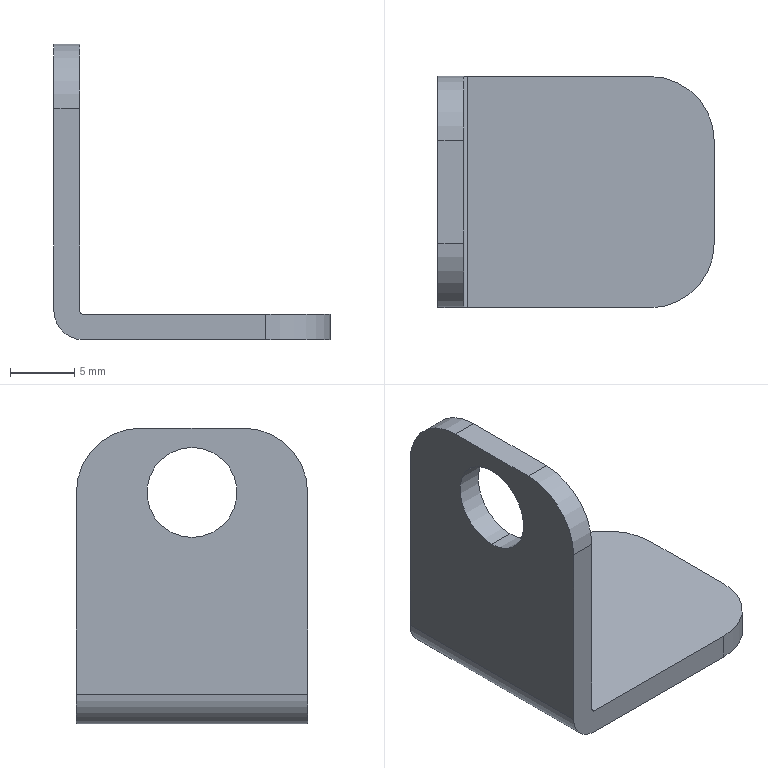Part | STEP file | Lower pull rod (lower door)_4 | 1 solid | 16 faces | box 21.5 x 18 x 23 mm | volume 1390 mm3 | cylinder 8 | plane 8 | commonest cylinder face diameters 10 x4 7 x2 0.6 x1 4.6 x1
STEP:
#1=CARTESIAN_POINT('',(0.,0.,0.));
#2=DIRECTION('',(0.,0.,1.));
#3=DIRECTION('',(1.,0.,0.));
#4=AXIS2_PLACEMENT_3D('',#1,#2,#3);
#5=CARTESIAN_POINT('',(217.,0.,23.5));
#6=VERTEX_POINT('',#5);
#7=CARTESIAN_POINT('',(215.,0.,23.5));
#8=VERTEX_POINT('',#7);
#9=CARTESIAN_POINT('',(217.,0.,23.5));
#10=DIRECTION('',(-1.,0.,0.));
#11=VECTOR('',#10,1.);
#12=LINE('',#9,#11);
#13=CARTESIAN_POINT('',(217.,0.,20.));
#14=DIRECTION('',(-1.,0.,0.));
#15=DIRECTION('',(0.,0.,1.));
#16=AXIS2_PLACEMENT_3D('',#13,#14,#15);
#17=CYLINDRICAL_SURFACE('',#16,3.5);
#18=CARTESIAN_POINT('',(6.283,0.));
#19=DIRECTION('',(0.,1.));
#20=VECTOR('',#19,1.);
#21=LINE('',#18,#20);
#22=(GEOMETRIC_REPRESENTATION_CONTEXT(2)PARAMETRIC_REPRESENTATION_CONTEXT()REPRESENTATION_CONTEXT('',''));
#23=DEFINITIONAL_REPRESENTATION('',(#21),#22);
#24=PCURVE('',#17,#23);
#25=CARTESIAN_POINT('',(217.,0.,20.));
#26=DIRECTION('',(-1.,0.,0.));
#27=DIRECTION('',(0.,0.,1.));
#28=AXIS2_PLACEMENT_3D('',#25,#26,#27);
#29=CYLINDRICAL_SURFACE('',#28,3.5);
#30=CARTESIAN_POINT('',(0.,0.));
#31=DIRECTION('',(0.,1.));
#32=VECTOR('',#31,1.);
#33=LINE('',#30,#32);
#34=(GEOMETRIC_REPRESENTATION_CONTEXT(2)PARAMETRIC_REPRESENTATION_CONTEXT()REPRESENTATION_CONTEXT('',''));
#35=DEFINITIONAL_REPRESENTATION('',(#33),#34);
#36=PCURVE('',#29,#35);
#37=SURFACE_CURVE('',#12,(#24,#36),.PCURVE_S1.);
#38=EDGE_CURVE('',#6,#8,#37,.T.);
#39=ORIENTED_EDGE('',*,*,#38,.T.);
#40=CARTESIAN_POINT('',(215.,0.,16.5));
#41=VERTEX_POINT('',#40);
#42=CARTESIAN_POINT('',(215.,0.,20.));
#43=DIRECTION('',(-1.,0.,0.));
#44=DIRECTION('',(0.,0.,1.));
#45=AXIS2_PLACEMENT_3D('',#42,#43,#44);
#46=CIRCLE('',#45,3.5);
#47=CARTESIAN_POINT('',(0.,2.));
#48=DIRECTION('',(1.,0.));
#49=VECTOR('',#48,1.);
#50=LINE('',#47,#49);
#51=(GEOMETRIC_REPRESENTATION_CONTEXT(2)PARAMETRIC_REPRESENTATION_CONTEXT()REPRESENTATION_CONTEXT('',''));
#52=DEFINITIONAL_REPRESENTATION('',(#50),#51);
#53=PCURVE('',#17,#52);
#54=CARTESIAN_POINT('',(215.,-9.,25.));
#55=DIRECTION('',(1.,0.,0.));
#56=DIRECTION('',(0.,0.,-1.));
#57=AXIS2_PLACEMENT_3D('',#54,#55,#56);
#58=PLANE('',#57);
#59=CARTESIAN_POINT('',(1.5,9.));
#60=CARTESIAN_POINT('',(1.5,15.062));
#61=CARTESIAN_POINT('',(6.75,12.031));
#62=CARTESIAN_POINT('',(12.,9.));
#63=CARTESIAN_POINT('',(6.75,5.969));
#64=CARTESIAN_POINT('',(1.5,2.938));
#65=CARTESIAN_POINT('',(1.5,9.));
#66=(BOUNDED_CURVE()B_SPLINE_CURVE(2,(#59,#60,#61,#62,#63,#64,#65),.UNSPECIFIED.,.T.,.F.)B_SPLINE_CURVE_WITH_KNOTS((1,2,2,2,2,1),(-2.094,0.,2.094,4.189,6.283,8.378),.UNSPECIFIED.)CURVE()GEOMETRIC_REPRESENTATION_ITEM()RATIONAL_B_SPLINE_CURVE((1.,0.5,1.,0.5,1.,0.5,1.))REPRESENTATION_ITEM(''));
#67=(GEOMETRIC_REPRESENTATION_CONTEXT(2)PARAMETRIC_REPRESENTATION_CONTEXT()REPRESENTATION_CONTEXT('',''));
#68=DEFINITIONAL_REPRESENTATION('',(#66),#67);
#69=PCURVE('',#58,#68);
#70=SURFACE_CURVE('',#46,(#53,#69),.PCURVE_S1.);
#71=EDGE_CURVE('',#41,#8,#70,.T.);
#72=ORIENTED_EDGE('',*,*,#71,.F.);
#73=CARTESIAN_POINT('',(217.,0.,16.5));
#74=VERTEX_POINT('',#73);
#75=CARTESIAN_POINT('',(217.,0.,16.5));
#76=DIRECTION('',(-1.,0.,0.));
#77=VECTOR('',#76,1.);
#78=LINE('',#75,#77);
#79=CARTESIAN_POINT('',(3.142,0.));
#80=DIRECTION('',(0.,1.));
#81=VECTOR('',#80,1.);
#82=LINE('',#79,#81);
#83=(GEOMETRIC_REPRESENTATION_CONTEXT(2)PARAMETRIC_REPRESENTATION_CONTEXT()REPRESENTATION_CONTEXT('',''));
#84=DEFINITIONAL_REPRESENTATION('',(#82),#83);
#85=PCURVE('',#17,#84);
#86=CARTESIAN_POINT('',(3.142,0.));
#87=DIRECTION('',(0.,1.));
#88=VECTOR('',#87,1.);
#89=LINE('',#86,#88);
#90=(GEOMETRIC_REPRESENTATION_CONTEXT(2)PARAMETRIC_REPRESENTATION_CONTEXT()REPRESENTATION_CONTEXT('',''));
#91=DEFINITIONAL_REPRESENTATION('',(#89),#90);
#92=PCURVE('',#29,#91);
#93=SURFACE_CURVE('',#78,(#85,#92),.PCURVE_S1.);
#94=EDGE_CURVE('',#74,#41,#93,.T.);
#95=ORIENTED_EDGE('',*,*,#94,.F.);
#96=CARTESIAN_POINT('',(217.,0.,20.));
#97=DIRECTION('',(-1.,0.,0.));
#98=DIRECTION('',(0.,0.,1.));
#99=AXIS2_PLACEMENT_3D('',#96,#97,#98);
#100=CIRCLE('',#99,3.5);
#101=CARTESIAN_POINT('',(0.,0.));
#102=DIRECTION('',(1.,0.));
#103=VECTOR('',#102,1.);
#104=LINE('',#101,#103);
#105=(GEOMETRIC_REPRESENTATION_CONTEXT(2)PARAMETRIC_REPRESENTATION_CONTEXT()REPRESENTATION_CONTEXT('',''));
#106=DEFINITIONAL_REPRESENTATION('',(#104),#105);
#107=PCURVE('',#17,#106);
#108=CARTESIAN_POINT('',(217.,-9.,25.));
#109=DIRECTION('',(1.,0.,0.));
#110=DIRECTION('',(0.,0.,-1.));
#111=AXIS2_PLACEMENT_3D('',#108,#109,#110);
#112=PLANE('',#111);
#113=CARTESIAN_POINT('',(1.5,9.));
#114=CARTESIAN_POINT('',(1.5,15.062));
#115=CARTESIAN_POINT('',(6.75,12.031));
#116=CARTESIAN_POINT('',(12.,9.));
#117=CARTESIAN_POINT('',(6.75,5.969));
#118=CARTESIAN_POINT('',(1.5,2.938));
#119=CARTESIAN_POINT('',(1.5,9.));
#120=(BOUNDED_CURVE()B_SPLINE_CURVE(2,(#113,#114,#115,#116,#117,#118,#119),.UNSPECIFIED.,.T.,.F.)B_SPLINE_CURVE_WITH_KNOTS((1,2,2,2,2,1),(-2.094,0.,2.094,4.189,6.283,8.378),.UNSPECIFIED.)CURVE()GEOMETRIC_REPRESENTATION_ITEM()RATIONAL_B_SPLINE_CURVE((1.,0.5,1.,0.5,1.,0.5,1.))REPRESENTATION_ITEM(''));
#121=(GEOMETRIC_REPRESENTATION_CONTEXT(2)PARAMETRIC_REPRESENTATION_CONTEXT()REPRESENTATION_CONTEXT('',''));
#122=DEFINITIONAL_REPRESENTATION('',(#120),#121);
#123=PCURVE('',#112,#122);
#124=SURFACE_CURVE('',#100,(#107,#123),.PCURVE_S1.);
#125=EDGE_CURVE('',#74,#6,#124,.T.);
#126=ORIENTED_EDGE('',*,*,#125,.T.);
#127=EDGE_LOOP('',(#39,#72,#95,#126));
#128=FACE_BOUND('',#127,.F.);
#129=ADVANCED_FACE('',(#128),#17,.F.);
#130=CARTESIAN_POINT('',(217.3,-9.,4.));
#131=VERTEX_POINT('',#130);
#132=CARTESIAN_POINT('',(231.5,-9.,4.));
#133=VERTEX_POINT('',#132);
#134=CARTESIAN_POINT('',(215.,-9.,4.));
#135=DIRECTION('',(1.,0.,0.));
#136=VECTOR('',#135,1.);
#137=LINE('',#134,#136);
#138=CARTESIAN_POINT('',(215.,-9.,4.));
#139=DIRECTION('',(0.,0.,1.));
#140=DIRECTION('',(1.,0.,0.));
#141=AXIS2_PLACEMENT_3D('',#138,#139,#140);
#142=PLANE('',#141);
#143=CARTESIAN_POINT('',(0.,0.));
#144=DIRECTION('',(1.,0.));
#145=VECTOR('',#144,1.);
#146=LINE('',#143,#145);
#147=(GEOMETRIC_REPRESENTATION_CONTEXT(2)PARAMETRIC_REPRESENTATION_CONTEXT()REPRESENTATION_CONTEXT('',''));
#148=DEFINITIONAL_REPRESENTATION('',(#146),#147);
#149=PCURVE('',#142,#148);
#150=CARTESIAN_POINT('',(217.3,-9.,4.3));
#151=DIRECTION('',(0.,1.,0.));
#152=DIRECTION('',(0.,0.,1.));
#153=AXIS2_PLACEMENT_3D('',#150,#151,#152);
#154=PLANE('',#153);
#155=CARTESIAN_POINT('',(-0.3,-2.3));
#156=DIRECTION('',(0.,1.));
#157=VECTOR('',#156,1.);
#158=LINE('',#155,#157);
#159=(GEOMETRIC_REPRESENTATION_CONTEXT(2)PARAMETRIC_REPRESENTATION_CONTEXT()REPRESENTATION_CONTEXT('',''));
#160=DEFINITIONAL_REPRESENTATION('',(#158),#159);
#161=PCURVE('',#154,#160);
#162=SURFACE_CURVE('',#137,(#149,#161),.PCURVE_S1.);
#163=EDGE_CURVE('',#131,#133,#162,.T.);
#164=ORIENTED_EDGE('',*,*,#163,.T.);
#165=CARTESIAN_POINT('',(236.5,-4.,4.));
#166=VERTEX_POINT('',#165);
#167=CARTESIAN_POINT('',(231.5,-4.,4.));
#168=DIRECTION('',(0.,0.,1.));
#169=DIRECTION('',(1.,0.,0.));
#170=AXIS2_PLACEMENT_3D('',#167,#168,#169);
#171=CIRCLE('',#170,5.);
#172=CARTESIAN_POINT('',(16.5,5.));
#173=DIRECTION('',(1.,0.));
#174=AXIS2_PLACEMENT_2D('',#172,#173);
#175=CIRCLE('',#174,5.);
#176=(GEOMETRIC_REPRESENTATION_CONTEXT(2)PARAMETRIC_REPRESENTATION_CONTEXT()REPRESENTATION_CONTEXT('',''));
#177=DEFINITIONAL_REPRESENTATION('',(#175),#176);
#178=PCURVE('',#142,#177);
#179=CARTESIAN_POINT('',(231.5,-4.,4.3));
#180=DIRECTION('',(0.,0.,1.));
#181=DIRECTION('',(1.,0.,0.));
#182=AXIS2_PLACEMENT_3D('',#179,#180,#181);
#183=CYLINDRICAL_SURFACE('',#182,5.);
#184=CARTESIAN_POINT('',(0.,-0.3));
#185=DIRECTION('',(1.,0.));
#186=VECTOR('',#185,1.);
#187=LINE('',#184,#186);
#188=(GEOMETRIC_REPRESENTATION_CONTEXT(2)PARAMETRIC_REPRESENTATION_CONTEXT()REPRESENTATION_CONTEXT('',''));
#189=DEFINITIONAL_REPRESENTATION('',(#187),#188);
#190=PCURVE('',#183,#189);
#191=SURFACE_CURVE('',#171,(#178,#190),.PCURVE_S1.);
#192=EDGE_CURVE('',#133,#166,#191,.T.);
#193=ORIENTED_EDGE('',*,*,#192,.T.);
#194=CARTESIAN_POINT('',(236.5,4.,4.));
#195=VERTEX_POINT('',#194);
#196=CARTESIAN_POINT('',(236.5,-9.,4.));
#197=DIRECTION('',(0.,1.,0.));
#198=VECTOR('',#197,1.);
#199=LINE('',#196,#198);
#200=CARTESIAN_POINT('',(21.5,0.));
#201=DIRECTION('',(0.,1.));
#202=VECTOR('',#201,1.);
#203=LINE('',#200,#202);
#204=(GEOMETRIC_REPRESENTATION_CONTEXT(2)PARAMETRIC_REPRESENTATION_CONTEXT()REPRESENTATION_CONTEXT('',''));
#205=DEFINITIONAL_REPRESENTATION('',(#203),#204);
#206=PCURVE('',#142,#205);
#207=CARTESIAN_POINT('',(236.5,-9.,2.));
#208=DIRECTION('',(-1.,0.,0.));
#209=DIRECTION('',(0.,0.,1.));
#210=AXIS2_PLACEMENT_3D('',#207,#208,#209);
#211=PLANE('',#210);
#212=CARTESIAN_POINT('',(2.,0.));
#213=DIRECTION('',(0.,1.));
#214=VECTOR('',#213,1.);
#215=LINE('',#212,#214);
#216=(GEOMETRIC_REPRESENTATION_CONTEXT(2)PARAMETRIC_REPRESENTATION_CONTEXT()REPRESENTATION_CONTEXT('',''));
#217=DEFINITIONAL_REPRESENTATION('',(#215),#216);
#218=PCURVE('',#211,#217);
#219=SURFACE_CURVE('',#199,(#206,#218),.PCURVE_S1.);
#220=EDGE_CURVE('',#166,#195,#219,.T.);
#221=ORIENTED_EDGE('',*,*,#220,.T.);
#222=CARTESIAN_POINT('',(231.5,9.,4.));
#223=VERTEX_POINT('',#222);
#224=CARTESIAN_POINT('',(231.5,4.,4.));
#225=DIRECTION('',(0.,0.,1.));
#226=DIRECTION('',(1.,0.,0.));
#227=AXIS2_PLACEMENT_3D('',#224,#225,#226);
#228=CIRCLE('',#227,5.);
#229=CARTESIAN_POINT('',(16.5,13.));
#230=DIRECTION('',(1.,0.));
#231=AXIS2_PLACEMENT_2D('',#229,#230);
#232=CIRCLE('',#231,5.);
#233=(GEOMETRIC_REPRESENTATION_CONTEXT(2)PARAMETRIC_REPRESENTATION_CONTEXT()REPRESENTATION_CONTEXT('',''));
#234=DEFINITIONAL_REPRESENTATION('',(#232),#233);
#235=PCURVE('',#142,#234);
#236=CARTESIAN_POINT('',(231.5,4.,2.));
#237=DIRECTION('',(0.,0.,-1.));
#238=DIRECTION('',(-1.,0.,0.));
#239=AXIS2_PLACEMENT_3D('',#236,#237,#238);
#240=CYLINDRICAL_SURFACE('',#239,5.);
#241=CARTESIAN_POINT('',(3.142,-2.));
#242=DIRECTION('',(-1.,0.));
#243=VECTOR('',#242,1.);
#244=LINE('',#241,#243);
#245=(GEOMETRIC_REPRESENTATION_CONTEXT(2)PARAMETRIC_REPRESENTATION_CONTEXT()REPRESENTATION_CONTEXT('',''));
#246=DEFINITIONAL_REPRESENTATION('',(#244),#245);
#247=PCURVE('',#240,#246);
#248=SURFACE_CURVE('',#228,(#235,#247),.PCURVE_S1.);
#249=EDGE_CURVE('',#195,#223,#248,.T.);
#250=ORIENTED_EDGE('',*,*,#249,.T.);
#251=CARTESIAN_POINT('',(217.3,9.,4.));
#252=VERTEX_POINT('',#251);
#253=CARTESIAN_POINT('',(215.,9.,4.));
#254=DIRECTION('',(1.,0.,0.));
#255=VECTOR('',#254,1.);
#256=LINE('',#253,#255);
#257=CARTESIAN_POINT('',(0.,18.));
#258=DIRECTION('',(1.,0.));
#259=VECTOR('',#258,1.);
#260=LINE('',#257,#259);
#261=(GEOMETRIC_REPRESENTATION_CONTEXT(2)PARAMETRIC_REPRESENTATION_CONTEXT()REPRESENTATION_CONTEXT('',''));
#262=DEFINITIONAL_REPRESENTATION('',(#260),#261);
#263=PCURVE('',#142,#262);
#264=CARTESIAN_POINT('',(217.3,9.,4.3));
#265=DIRECTION('',(0.,1.,0.));
#266=DIRECTION('',(0.,0.,1.));
#267=AXIS2_PLACEMENT_3D('',#264,#265,#266);
#268=PLANE('',#267);
#269=CARTESIAN_POINT('',(-0.3,-2.3));
#270=DIRECTION('',(0.,1.));
#271=VECTOR('',#270,1.);
#272=LINE('',#269,#271);
#273=(GEOMETRIC_REPRESENTATION_CONTEXT(2)PARAMETRIC_REPRESENTATION_CONTEXT()REPRESENTATION_CONTEXT('',''));
#274=DEFINITIONAL_REPRESENTATION('',(#272),#273);
#275=PCURVE('',#268,#274);
#276=SURFACE_CURVE('',#256,(#263,#275),.PCURVE_S1.);
#277=EDGE_CURVE('',#252,#223,#276,.T.);
#278=ORIENTED_EDGE('',*,*,#277,.F.);
#279=CARTESIAN_POINT('',(217.3,-9.,4.));
#280=DIRECTION('',(0.,1.,0.));
#281=VECTOR('',#280,1.);
#282=LINE('',#279,#281);
#283=CARTESIAN_POINT('',(2.3,0.));
#284=DIRECTION('',(0.,1.));
#285=VECTOR('',#284,1.);
#286=LINE('',#283,#285);
#287=(GEOMETRIC_REPRESENTATION_CONTEXT(2)PARAMETRIC_REPRESENTATION_CONTEXT()REPRESENTATION_CONTEXT('',''));
#288=DEFINITIONAL_REPRESENTATION('',(#286),#287);
#289=PCURVE('',#142,#288);
#290=CARTESIAN_POINT('',(217.3,-9.,4.3));
#291=DIRECTION('',(0.,1.,0.));
#292=DIRECTION('',(0.,0.,1.));
#293=AXIS2_PLACEMENT_3D('',#290,#291,#292);
#294=CYLINDRICAL_SURFACE('',#293,0.3);
#295=CARTESIAN_POINT('',(3.142,0.));
#296=DIRECTION('',(0.,1.));
#297=VECTOR('',#296,1.);
#298=LINE('',#295,#297);
#299=(GEOMETRIC_REPRESENTATION_CONTEXT(2)PARAMETRIC_REPRESENTATION_CONTEXT()REPRESENTATION_CONTEXT('',''));
#300=DEFINITIONAL_REPRESENTATION('',(#298),#299);
#301=PCURVE('',#294,#300);
#302=SURFACE_CURVE('',#282,(#289,#301),.PCURVE_S1.);
#303=EDGE_CURVE('',#131,#252,#302,.T.);
#304=ORIENTED_EDGE('',*,*,#303,.F.);
#305=EDGE_LOOP('',(#164,#193,#221,#250,#278,#304));
#306=FACE_BOUND('',#305,.T.);
#307=ADVANCED_FACE('',(#306),#142,.T.);
#308=ORIENTED_EDGE('',*,*,#303,.F.);
#309=CARTESIAN_POINT('',(217.,-9.,4.3));
#310=VERTEX_POINT('',#309);
#311=CARTESIAN_POINT('',(217.3,-9.,4.3));
#312=DIRECTION('',(0.,-1.,0.));
#313=DIRECTION('',(-1.,0.,0.));
#314=AXIS2_PLACEMENT_3D('',#311,#312,#313);
#315=CIRCLE('',#314,0.3);
#316=CARTESIAN_POINT('',(4.712,0.));
#317=DIRECTION('',(-1.,0.));
#318=VECTOR('',#317,1.);
#319=LINE('',#316,#318);
#320=(GEOMETRIC_REPRESENTATION_CONTEXT(2)PARAMETRIC_REPRESENTATION_CONTEXT()REPRESENTATION_CONTEXT('',''));
#321=DEFINITIONAL_REPRESENTATION('',(#319),#320);
#322=PCURVE('',#294,#321);
#323=CARTESIAN_POINT('',(0.,-0.3));
#324=CARTESIAN_POINT('',(-0.5196,-0.3));
#325=CARTESIAN_POINT('',(-0.2598,0.15));
#326=CARTESIAN_POINT('',(0.,0.6));
#327=CARTESIAN_POINT('',(0.2598,0.15));
#328=CARTESIAN_POINT('',(0.5196,-0.3));
#329=CARTESIAN_POINT('',(0.,-0.3));
#330=(BOUNDED_CURVE()B_SPLINE_CURVE(2,(#323,#324,#325,#326,#327,#328,#329),.UNSPECIFIED.,.T.,.F.)B_SPLINE_CURVE_WITH_KNOTS((1,2,2,2,2,1),(-2.094,0.,2.094,4.189,6.283,8.378),.UNSPECIFIED.)CURVE()GEOMETRIC_REPRESENTATION_ITEM()RATIONAL_B_SPLINE_CURVE((1.,0.5,1.,0.5,1.,0.5,1.))REPRESENTATION_ITEM(''));
#331=(GEOMETRIC_REPRESENTATION_CONTEXT(2)PARAMETRIC_REPRESENTATION_CONTEXT()REPRESENTATION_CONTEXT('',''));
#332=DEFINITIONAL_REPRESENTATION('',(#330),#331);
#333=PCURVE('',#154,#332);
#334=SURFACE_CURVE('',#315,(#322,#333),.PCURVE_S1.);
#335=EDGE_CURVE('',#310,#131,#334,.T.);
#336=ORIENTED_EDGE('',*,*,#335,.F.);
#337=CARTESIAN_POINT('',(217.,9.,4.3));
#338=VERTEX_POINT('',#337);
#339=CARTESIAN_POINT('',(217.,-9.,4.3));
#340=DIRECTION('',(0.,1.,0.));
#341=VECTOR('',#340,1.);
#342=LINE('',#339,#341);
#343=CARTESIAN_POINT('',(4.712,0.));
#344=DIRECTION('',(0.,1.));
#345=VECTOR('',#344,1.);
#346=LINE('',#343,#345);
#347=(GEOMETRIC_REPRESENTATION_CONTEXT(2)PARAMETRIC_REPRESENTATION_CONTEXT()REPRESENTATION_CONTEXT('',''));
#348=DEFINITIONAL_REPRESENTATION('',(#346),#347);
#349=PCURVE('',#294,#348);
#350=CARTESIAN_POINT('',(20.7,0.));
#351=DIRECTION('',(0.,1.));
#352=VECTOR('',#351,1.);
#353=LINE('',#350,#352);
#354=(GEOMETRIC_REPRESENTATION_CONTEXT(2)PARAMETRIC_REPRESENTATION_CONTEXT()REPRESENTATION_CONTEXT('',''));
#355=DEFINITIONAL_REPRESENTATION('',(#353),#354);
#356=PCURVE('',#112,#355);
#357=SURFACE_CURVE('',#342,(#349,#356),.PCURVE_S1.);
#358=EDGE_CURVE('',#310,#338,#357,.T.);
#359=ORIENTED_EDGE('',*,*,#358,.T.);
#360=CARTESIAN_POINT('',(217.3,9.,4.3));
#361=DIRECTION('',(0.,-1.,0.));
#362=DIRECTION('',(-1.,0.,0.));
#363=AXIS2_PLACEMENT_3D('',#360,#361,#362);
#364=CIRCLE('',#363,0.3);
#365=CARTESIAN_POINT('',(4.712,18.));
#366=DIRECTION('',(-1.,0.));
#367=VECTOR('',#366,1.);
#368=LINE('',#365,#367);
#369=(GEOMETRIC_REPRESENTATION_CONTEXT(2)PARAMETRIC_REPRESENTATION_CONTEXT()REPRESENTATION_CONTEXT('',''));
#370=DEFINITIONAL_REPRESENTATION('',(#368),#369);
#371=PCURVE('',#294,#370);
#372=CARTESIAN_POINT('',(0.,-0.3));
#373=CARTESIAN_POINT('',(-0.5196,-0.3));
#374=CARTESIAN_POINT('',(-0.2598,0.15));
#375=CARTESIAN_POINT('',(0.,0.6));
#376=CARTESIAN_POINT('',(0.2598,0.15));
#377=CARTESIAN_POINT('',(0.5196,-0.3));
#378=CARTESIAN_POINT('',(0.,-0.3));
#379=(BOUNDED_CURVE()B_SPLINE_CURVE(2,(#372,#373,#374,#375,#376,#377,#378),.UNSPECIFIED.,.T.,.F.)B_SPLINE_CURVE_WITH_KNOTS((1,2,2,2,2,1),(-2.094,0.,2.094,4.189,6.283,8.378),.UNSPECIFIED.)CURVE()GEOMETRIC_REPRESENTATION_ITEM()RATIONAL_B_SPLINE_CURVE((1.,0.5,1.,0.5,1.,0.5,1.))REPRESENTATION_ITEM(''));
#380=(GEOMETRIC_REPRESENTATION_CONTEXT(2)PARAMETRIC_REPRESENTATION_CONTEXT()REPRESENTATION_CONTEXT('',''));
#381=DEFINITIONAL_REPRESENTATION('',(#379),#380);
#382=PCURVE('',#268,#381);
#383=SURFACE_CURVE('',#364,(#371,#382),.PCURVE_S1.);
#384=EDGE_CURVE('',#338,#252,#383,.T.);
#385=ORIENTED_EDGE('',*,*,#384,.T.);
#386=EDGE_LOOP('',(#308,#336,#359,#385));
#387=FACE_BOUND('',#386,.F.);
#388=ADVANCED_FACE('',(#387),#294,.F.);
#389=CARTESIAN_POINT('',(217.,0.,20.));
#390=DIRECTION('',(-1.,0.,0.));
#391=DIRECTION('',(0.,0.,1.));
#392=AXIS2_PLACEMENT_3D('',#389,#390,#391);
#393=CIRCLE('',#392,3.5);
#394=CARTESIAN_POINT('',(1.5,9.));
#395=CARTESIAN_POINT('',(1.5,15.062));
#396=CARTESIAN_POINT('',(6.75,12.031));
#397=CARTESIAN_POINT('',(12.,9.));
#398=CARTESIAN_POINT('',(6.75,5.969));
#399=CARTESIAN_POINT('',(1.5,2.938));
#400=CARTESIAN_POINT('',(1.5,9.));
#401=(BOUNDED_CURVE()B_SPLINE_CURVE(2,(#394,#395,#396,#397,#398,#399,#400),.UNSPECIFIED.,.T.,.F.)B_SPLINE_CURVE_WITH_KNOTS((1,2,2,2,2,1),(-2.094,0.,2.094,4.189,6.283,8.378),.UNSPECIFIED.)CURVE()GEOMETRIC_REPRESENTATION_ITEM()RATIONAL_B_SPLINE_CURVE((1.,0.5,1.,0.5,1.,0.5,1.))REPRESENTATION_ITEM(''));
#402=(GEOMETRIC_REPRESENTATION_CONTEXT(2)PARAMETRIC_REPRESENTATION_CONTEXT()REPRESENTATION_CONTEXT('',''));
#403=DEFINITIONAL_REPRESENTATION('',(#401),#402);
#404=PCURVE('',#112,#403);
#405=CARTESIAN_POINT('',(0.,0.));
#406=DIRECTION('',(1.,0.));
#407=VECTOR('',#406,1.);
#408=LINE('',#405,#407);
#409=(GEOMETRIC_REPRESENTATION_CONTEXT(2)PARAMETRIC_REPRESENTATION_CONTEXT()REPRESENTATION_CONTEXT('',''));
#410=DEFINITIONAL_REPRESENTATION('',(#408),#409);
#411=PCURVE('',#29,#410);
#412=SURFACE_CURVE('',#393,(#404,#411),.PCURVE_S1.);
#413=EDGE_CURVE('',#6,#74,#412,.T.);
#414=ORIENTED_EDGE('',*,*,#413,.T.);
#415=ORIENTED_EDGE('',*,*,#125,.T.);
#416=EDGE_LOOP('',(#414,#415));
#417=FACE_BOUND('',#416,.T.);
#418=CARTESIAN_POINT('',(217.,-4.,25.));
#419=VERTEX_POINT('',#418);
#420=CARTESIAN_POINT('',(217.,4.,25.));
#421=VERTEX_POINT('',#420);
#422=CARTESIAN_POINT('',(217.,-9.,25.));
#423=DIRECTION('',(0.,1.,0.));
#424=VECTOR('',#423,1.);
#425=LINE('',#422,#424);
#426=CARTESIAN_POINT('',(0.,0.));
#427=DIRECTION('',(0.,1.));
#428=VECTOR('',#427,1.);
#429=LINE('',#426,#428);
#430=(GEOMETRIC_REPRESENTATION_CONTEXT(2)PARAMETRIC_REPRESENTATION_CONTEXT()REPRESENTATION_CONTEXT('',''));
#431=DEFINITIONAL_REPRESENTATION('',(#429),#430);
#432=PCURVE('',#112,#431);
#433=CARTESIAN_POINT('',(217.,-9.,25.));
#434=DIRECTION('',(0.,0.,-1.));
#435=DIRECTION('',(-1.,0.,0.));
#436=AXIS2_PLACEMENT_3D('',#433,#434,#435);
#437=PLANE('',#436);
#438=CARTESIAN_POINT('',(0.,0.));
#439=DIRECTION('',(0.,1.));
#440=VECTOR('',#439,1.);
#441=LINE('',#438,#440);
#442=(GEOMETRIC_REPRESENTATION_CONTEXT(2)PARAMETRIC_REPRESENTATION_CONTEXT()REPRESENTATION_CONTEXT('',''));
#443=DEFINITIONAL_REPRESENTATION('',(#441),#442);
#444=PCURVE('',#437,#443);
#445=SURFACE_CURVE('',#425,(#432,#444),.PCURVE_S1.);
#446=EDGE_CURVE('',#419,#421,#445,.T.);
#447=ORIENTED_EDGE('',*,*,#446,.F.);
#448=CARTESIAN_POINT('',(217.,-9.,20.));
#449=VERTEX_POINT('',#448);
#450=CARTESIAN_POINT('',(217.,-4.,20.));
#451=DIRECTION('',(1.,0.,0.));
#452=DIRECTION('',(0.,0.,-1.));
#453=AXIS2_PLACEMENT_3D('',#450,#451,#452);
#454=CIRCLE('',#453,5.);
#455=CARTESIAN_POINT('',(5.,5.));
#456=DIRECTION('',(1.,0.));
#457=AXIS2_PLACEMENT_2D('',#455,#456);
#458=CIRCLE('',#457,5.);
#459=(GEOMETRIC_REPRESENTATION_CONTEXT(2)PARAMETRIC_REPRESENTATION_CONTEXT()REPRESENTATION_CONTEXT('',''));
#460=DEFINITIONAL_REPRESENTATION('',(#458),#459);
#461=PCURVE('',#112,#460);
#462=CARTESIAN_POINT('',(217.3,-4.,20.));
#463=DIRECTION('',(1.,0.,0.));
#464=DIRECTION('',(0.,0.,-1.));
#465=AXIS2_PLACEMENT_3D('',#462,#463,#464);
#466=CYLINDRICAL_SURFACE('',#465,5.);
#467=CARTESIAN_POINT('',(0.,-0.3));
#468=DIRECTION('',(1.,0.));
#469=VECTOR('',#468,1.);
#470=LINE('',#467,#469);
#471=(GEOMETRIC_REPRESENTATION_CONTEXT(2)PARAMETRIC_REPRESENTATION_CONTEXT()REPRESENTATION_CONTEXT('',''));
#472=DEFINITIONAL_REPRESENTATION('',(#470),#471);
#473=PCURVE('',#466,#472);
#474=SURFACE_CURVE('',#454,(#461,#473),.PCURVE_S1.);
#475=EDGE_CURVE('',#419,#449,#474,.T.);
#476=ORIENTED_EDGE('',*,*,#475,.T.);
#477=CARTESIAN_POINT('',(217.,-9.,25.));
#478=DIRECTION('',(0.,0.,-1.));
#479=VECTOR('',#478,1.);
#480=LINE('',#477,#479);
#481=CARTESIAN_POINT('',(0.,0.));
#482=DIRECTION('',(1.,0.));
#483=VECTOR('',#482,1.);
#484=LINE('',#481,#483);
#485=(GEOMETRIC_REPRESENTATION_CONTEXT(2)PARAMETRIC_REPRESENTATION_CONTEXT()REPRESENTATION_CONTEXT('',''));
#486=DEFINITIONAL_REPRESENTATION('',(#484),#485);
#487=PCURVE('',#112,#486);
#488=CARTESIAN_POINT('',(20.7,-0.3));
#489=DIRECTION('',(-1.,0.));
#490=VECTOR('',#489,1.);
#491=LINE('',#488,#490);
#492=(GEOMETRIC_REPRESENTATION_CONTEXT(2)PARAMETRIC_REPRESENTATION_CONTEXT()REPRESENTATION_CONTEXT('',''));
#493=DEFINITIONAL_REPRESENTATION('',(#491),#492);
#494=PCURVE('',#154,#493);
#495=SURFACE_CURVE('',#480,(#487,#494),.PCURVE_S1.);
#496=EDGE_CURVE('',#449,#310,#495,.T.);
#497=ORIENTED_EDGE('',*,*,#496,.T.);
#498=ORIENTED_EDGE('',*,*,#358,.T.);
#499=CARTESIAN_POINT('',(217.,9.,20.));
#500=VERTEX_POINT('',#499);
#501=CARTESIAN_POINT('',(217.,9.,25.));
#502=DIRECTION('',(0.,0.,-1.));
#503=VECTOR('',#502,1.);
#504=LINE('',#501,#503);
#505=CARTESIAN_POINT('',(0.,18.));
#506=DIRECTION('',(1.,0.));
#507=VECTOR('',#506,1.);
#508=LINE('',#505,#507);
#509=(GEOMETRIC_REPRESENTATION_CONTEXT(2)PARAMETRIC_REPRESENTATION_CONTEXT()REPRESENTATION_CONTEXT('',''));
#510=DEFINITIONAL_REPRESENTATION('',(#508),#509);
#511=PCURVE('',#112,#510);
#512=CARTESIAN_POINT('',(20.7,-0.3));
#513=DIRECTION('',(-1.,0.));
#514=VECTOR('',#513,1.);
#515=LINE('',#512,#514);
#516=(GEOMETRIC_REPRESENTATION_CONTEXT(2)PARAMETRIC_REPRESENTATION_CONTEXT()REPRESENTATION_CONTEXT('',''));
#517=DEFINITIONAL_REPRESENTATION('',(#515),#516);
#518=PCURVE('',#268,#517);
#519=SURFACE_CURVE('',#504,(#511,#518),.PCURVE_S1.);
#520=EDGE_CURVE('',#500,#338,#519,.T.);
#521=ORIENTED_EDGE('',*,*,#520,.F.);
#522=CARTESIAN_POINT('',(217.,4.,20.));
#523=DIRECTION('',(1.,0.,0.));
#524=DIRECTION('',(0.,0.,-1.));
#525=AXIS2_PLACEMENT_3D('',#522,#523,#524);
#526=CIRCLE('',#525,5.);
#527=CARTESIAN_POINT('',(5.,13.));
#528=DIRECTION('',(1.,0.));
#529=AXIS2_PLACEMENT_2D('',#527,#528);
#530=CIRCLE('',#529,5.);
#531=(GEOMETRIC_REPRESENTATION_CONTEXT(2)PARAMETRIC_REPRESENTATION_CONTEXT()REPRESENTATION_CONTEXT('',''));
#532=DEFINITIONAL_REPRESENTATION('',(#530),#531);
#533=PCURVE('',#112,#532);
#534=CARTESIAN_POINT('',(217.,4.,20.));
#535=DIRECTION('',(1.,0.,0.));
#536=DIRECTION('',(0.,0.,-1.));
#537=AXIS2_PLACEMENT_3D('',#534,#535,#536);
#538=CYLINDRICAL_SURFACE('',#537,5.);
#539=CARTESIAN_POINT('',(0.,0.));
#540=DIRECTION('',(1.,0.));
#541=VECTOR('',#540,1.);
#542=LINE('',#539,#541);
#543=(GEOMETRIC_REPRESENTATION_CONTEXT(2)PARAMETRIC_REPRESENTATION_CONTEXT()REPRESENTATION_CONTEXT('',''));
#544=DEFINITIONAL_REPRESENTATION('',(#542),#543);
#545=PCURVE('',#538,#544);
#546=SURFACE_CURVE('',#526,(#533,#545),.PCURVE_S1.);
#547=EDGE_CURVE('',#500,#421,#546,.T.);
#548=ORIENTED_EDGE('',*,*,#547,.T.);
#549=EDGE_LOOP('',(#447,#476,#497,#498,#521,#548));
#550=FACE_BOUND('',#549,.T.);
#551=ADVANCED_FACE('',(#417,#550),#112,.T.);
#552=CARTESIAN_POINT('',(215.,-4.,25.));
#553=VERTEX_POINT('',#552);
#554=CARTESIAN_POINT('',(215.,4.,25.));
#555=VERTEX_POINT('',#554);
#556=CARTESIAN_POINT('',(215.,-9.,25.));
#557=DIRECTION('',(0.,1.,0.));
#558=VECTOR('',#557,1.);
#559=LINE('',#556,#558);
#560=CARTESIAN_POINT('',(2.,0.));
#561=DIRECTION('',(0.,1.));
#562=VECTOR('',#561,1.);
#563=LINE('',#560,#562);
#564=(GEOMETRIC_REPRESENTATION_CONTEXT(2)PARAMETRIC_REPRESENTATION_CONTEXT()REPRESENTATION_CONTEXT('',''));
#565=DEFINITIONAL_REPRESENTATION('',(#563),#564);
#566=PCURVE('',#437,#565);
#567=CARTESIAN_POINT('',(0.,0.));
#568=DIRECTION('',(0.,1.));
#569=VECTOR('',#568,1.);
#570=LINE('',#567,#569);
#571=(GEOMETRIC_REPRESENTATION_CONTEXT(2)PARAMETRIC_REPRESENTATION_CONTEXT()REPRESENTATION_CONTEXT('',''));
#572=DEFINITIONAL_REPRESENTATION('',(#570),#571);
#573=PCURVE('',#58,#572);
#574=SURFACE_CURVE('',#559,(#566,#573),.PCURVE_S1.);
#575=EDGE_CURVE('',#553,#555,#574,.T.);
#576=ORIENTED_EDGE('',*,*,#575,.F.);
#577=CARTESIAN_POINT('',(217.,-4.,25.));
#578=DIRECTION('',(1.,0.,0.));
#579=VECTOR('',#578,1.);
#580=LINE('',#577,#579);
#581=CARTESIAN_POINT('',(0.,5.));
#582=DIRECTION('',(-1.,0.));
#583=VECTOR('',#582,1.);
#584=LINE('',#581,#583);
#585=(GEOMETRIC_REPRESENTATION_CONTEXT(2)PARAMETRIC_REPRESENTATION_CONTEXT()REPRESENTATION_CONTEXT('',''));
#586=DEFINITIONAL_REPRESENTATION('',(#584),#585);
#587=PCURVE('',#437,#586);
#588=CARTESIAN_POINT('',(3.142,-0.3));
#589=DIRECTION('',(0.,1.));
#590=VECTOR('',#589,1.);
#591=LINE('',#588,#590);
#592=(GEOMETRIC_REPRESENTATION_CONTEXT(2)PARAMETRIC_REPRESENTATION_CONTEXT()REPRESENTATION_CONTEXT('',''));
#593=DEFINITIONAL_REPRESENTATION('',(#591),#592);
#594=PCURVE('',#466,#593);
#595=SURFACE_CURVE('',#580,(#587,#594),.PCURVE_S1.);
#596=EDGE_CURVE('',#553,#419,#595,.T.);
#597=ORIENTED_EDGE('',*,*,#596,.T.);
#598=ORIENTED_EDGE('',*,*,#446,.T.);
#599=CARTESIAN_POINT('',(215.,4.,25.));
#600=DIRECTION('',(-1.,0.,0.));
#601=VECTOR('',#600,1.);
#602=LINE('',#599,#601);
#603=CARTESIAN_POINT('',(2.,13.));
#604=DIRECTION('',(1.,0.));
#605=VECTOR('',#604,1.);
#606=LINE('',#603,#605);
#607=(GEOMETRIC_REPRESENTATION_CONTEXT(2)PARAMETRIC_REPRESENTATION_CONTEXT()REPRESENTATION_CONTEXT('',''));
#608=DEFINITIONAL_REPRESENTATION('',(#606),#607);
#609=PCURVE('',#437,#608);
#610=CARTESIAN_POINT('',(3.142,-2.));
#611=DIRECTION('',(0.,-1.));
#612=VECTOR('',#611,1.);
#613=LINE('',#610,#612);
#614=(GEOMETRIC_REPRESENTATION_CONTEXT(2)PARAMETRIC_REPRESENTATION_CONTEXT()REPRESENTATION_CONTEXT('',''));
#615=DEFINITIONAL_REPRESENTATION('',(#613),#614);
#616=PCURVE('',#538,#615);
#617=SURFACE_CURVE('',#602,(#609,#616),.PCURVE_S1.);
#618=EDGE_CURVE('',#421,#555,#617,.T.);
#619=ORIENTED_EDGE('',*,*,#618,.T.);
#620=EDGE_LOOP('',(#576,#597,#598,#619));
#621=FACE_BOUND('',#620,.T.);
#622=ADVANCED_FACE('',(#621),#437,.F.);
#623=CARTESIAN_POINT('',(215.,0.,20.));
#624=DIRECTION('',(-1.,0.,0.));
#625=DIRECTION('',(0.,0.,1.));
#626=AXIS2_PLACEMENT_3D('',#623,#624,#625);
#627=CIRCLE('',#626,3.5);
#628=CARTESIAN_POINT('',(1.5,9.));
#629=CARTESIAN_POINT('',(1.5,15.062));
#630=CARTESIAN_POINT('',(6.75,12.031));
#631=CARTESIAN_POINT('',(12.,9.));
#632=CARTESIAN_POINT('',(6.75,5.969));
#633=CARTESIAN_POINT('',(1.5,2.938));
#634=CARTESIAN_POINT('',(1.5,9.));
#635=(BOUNDED_CURVE()B_SPLINE_CURVE(2,(#628,#629,#630,#631,#632,#633,#634),.UNSPECIFIED.,.T.,.F.)B_SPLINE_CURVE_WITH_KNOTS((1,2,2,2,2,1),(-2.094,0.,2.094,4.189,6.283,8.378),.UNSPECIFIED.)CURVE()GEOMETRIC_REPRESENTATION_ITEM()RATIONAL_B_SPLINE_CURVE((1.,0.5,1.,0.5,1.,0.5,1.))REPRESENTATION_ITEM(''));
#636=(GEOMETRIC_REPRESENTATION_CONTEXT(2)PARAMETRIC_REPRESENTATION_CONTEXT()REPRESENTATION_CONTEXT('',''));
#637=DEFINITIONAL_REPRESENTATION('',(#635),#636);
#638=PCURVE('',#58,#637);
#639=CARTESIAN_POINT('',(0.,2.));
#640=DIRECTION('',(1.,0.));
#641=VECTOR('',#640,1.);
#642=LINE('',#639,#641);
#643=(GEOMETRIC_REPRESENTATION_CONTEXT(2)PARAMETRIC_REPRESENTATION_CONTEXT()REPRESENTATION_CONTEXT('',''));
#644=DEFINITIONAL_REPRESENTATION('',(#642),#643);
#645=PCURVE('',#29,#644);
#646=SURFACE_CURVE('',#627,(#638,#645),.PCURVE_S1.);
#647=EDGE_CURVE('',#8,#41,#646,.T.);
#648=ORIENTED_EDGE('',*,*,#647,.F.);
#649=ORIENTED_EDGE('',*,*,#71,.F.);
#650=EDGE_LOOP('',(#648,#649));
#651=FACE_BOUND('',#650,.T.);
#652=CARTESIAN_POINT('',(215.,-9.,20.));
#653=VERTEX_POINT('',#652);
#654=CARTESIAN_POINT('',(215.,-9.,4.3));
#655=VERTEX_POINT('',#654);
#656=CARTESIAN_POINT('',(215.,-9.,25.));
#657=DIRECTION('',(0.,0.,-1.));
#658=VECTOR('',#657,1.);
#659=LINE('',#656,#658);
#660=CARTESIAN_POINT('',(0.,0.));
#661=DIRECTION('',(1.,0.));
#662=VECTOR('',#661,1.);
#663=LINE('',#660,#662);
#664=(GEOMETRIC_REPRESENTATION_CONTEXT(2)PARAMETRIC_REPRESENTATION_CONTEXT()REPRESENTATION_CONTEXT('',''));
#665=DEFINITIONAL_REPRESENTATION('',(#663),#664);
#666=PCURVE('',#58,#665);
#667=CARTESIAN_POINT('',(20.7,-2.3));
#668=DIRECTION('',(-1.,0.));
#669=VECTOR('',#668,1.);
#670=LINE('',#667,#669);
#671=(GEOMETRIC_REPRESENTATION_CONTEXT(2)PARAMETRIC_REPRESENTATION_CONTEXT()REPRESENTATION_CONTEXT('',''));
#672=DEFINITIONAL_REPRESENTATION('',(#670),#671);
#673=PCURVE('',#154,#672);
#674=SURFACE_CURVE('',#659,(#666,#673),.PCURVE_S1.);
#675=EDGE_CURVE('',#653,#655,#674,.T.);
#676=ORIENTED_EDGE('',*,*,#675,.F.);
#677=CARTESIAN_POINT('',(215.,-4.,20.));
#678=DIRECTION('',(-1.,0.,0.));
#679=DIRECTION('',(0.,0.,-1.));
#680=AXIS2_PLACEMENT_3D('',#677,#678,#679);
#681=CIRCLE('',#680,5.);
#682=CARTESIAN_POINT('',(10.,5.));
#683=CARTESIAN_POINT('',(10.,-3.66));
#684=CARTESIAN_POINT('',(2.5,0.6699));
#685=CARTESIAN_POINT('',(-5.,5.));
#686=CARTESIAN_POINT('',(2.5,9.33));
#687=CARTESIAN_POINT('',(10.,13.66));
#688=CARTESIAN_POINT('',(10.,5.));
#689=(BOUNDED_CURVE()B_SPLINE_CURVE(2,(#682,#683,#684,#685,#686,#687,#688),.UNSPECIFIED.,.T.,.F.)B_SPLINE_CURVE_WITH_KNOTS((1,2,2,2,2,1),(-2.094,0.,2.094,4.189,6.283,8.378),.UNSPECIFIED.)CURVE()GEOMETRIC_REPRESENTATION_ITEM()RATIONAL_B_SPLINE_CURVE((1.,0.5,1.,0.5,1.,0.5,1.))REPRESENTATION_ITEM(''));
#690=(GEOMETRIC_REPRESENTATION_CONTEXT(2)PARAMETRIC_REPRESENTATION_CONTEXT()REPRESENTATION_CONTEXT('',''));
#691=DEFINITIONAL_REPRESENTATION('',(#689),#690);
#692=PCURVE('',#58,#691);
#693=CARTESIAN_POINT('',(6.283,-2.3));
#694=DIRECTION('',(-1.,0.));
#695=VECTOR('',#694,1.);
#696=LINE('',#693,#695);
#697=(GEOMETRIC_REPRESENTATION_CONTEXT(2)PARAMETRIC_REPRESENTATION_CONTEXT()REPRESENTATION_CONTEXT('',''));
#698=DEFINITIONAL_REPRESENTATION('',(#696),#697);
#699=PCURVE('',#466,#698);
#700=SURFACE_CURVE('',#681,(#692,#699),.PCURVE_S1.);
#701=EDGE_CURVE('',#653,#553,#700,.T.);
#702=ORIENTED_EDGE('',*,*,#701,.T.);
#703=ORIENTED_EDGE('',*,*,#575,.T.);
#704=CARTESIAN_POINT('',(215.,9.,20.));
#705=VERTEX_POINT('',#704);
#706=CARTESIAN_POINT('',(215.,4.,20.));
#707=DIRECTION('',(-1.,0.,0.));
#708=DIRECTION('',(0.,0.,-1.));
#709=AXIS2_PLACEMENT_3D('',#706,#707,#708);
#710=CIRCLE('',#709,5.);
#711=CARTESIAN_POINT('',(10.,13.));
#712=CARTESIAN_POINT('',(10.,4.34));
#713=CARTESIAN_POINT('',(2.5,8.67));
#714=CARTESIAN_POINT('',(-5.,13.));
#715=CARTESIAN_POINT('',(2.5,17.33));
#716=CARTESIAN_POINT('',(10.,21.66));
#717=CARTESIAN_POINT('',(10.,13.));
#718=(BOUNDED_CURVE()B_SPLINE_CURVE(2,(#711,#712,#713,#714,#715,#716,#717),.UNSPECIFIED.,.T.,.F.)B_SPLINE_CURVE_WITH_KNOTS((1,2,2,2,2,1),(-2.094,0.,2.094,4.189,6.283,8.378),.UNSPECIFIED.)CURVE()GEOMETRIC_REPRESENTATION_ITEM()RATIONAL_B_SPLINE_CURVE((1.,0.5,1.,0.5,1.,0.5,1.))REPRESENTATION_ITEM(''));
#719=(GEOMETRIC_REPRESENTATION_CONTEXT(2)PARAMETRIC_REPRESENTATION_CONTEXT()REPRESENTATION_CONTEXT('',''));
#720=DEFINITIONAL_REPRESENTATION('',(#718),#719);
#721=PCURVE('',#58,#720);
#722=CARTESIAN_POINT('',(6.283,-2.));
#723=DIRECTION('',(-1.,0.));
#724=VECTOR('',#723,1.);
#725=LINE('',#722,#724);
#726=(GEOMETRIC_REPRESENTATION_CONTEXT(2)PARAMETRIC_REPRESENTATION_CONTEXT()REPRESENTATION_CONTEXT('',''));
#727=DEFINITIONAL_REPRESENTATION('',(#725),#726);
#728=PCURVE('',#538,#727);
#729=SURFACE_CURVE('',#710,(#721,#728),.PCURVE_S1.);
#730=EDGE_CURVE('',#555,#705,#729,.T.);
#731=ORIENTED_EDGE('',*,*,#730,.T.);
#732=CARTESIAN_POINT('',(215.,9.,4.3));
#733=VERTEX_POINT('',#732);
#734=CARTESIAN_POINT('',(215.,9.,25.));
#735=DIRECTION('',(0.,0.,-1.));
#736=VECTOR('',#735,1.);
#737=LINE('',#734,#736);
#738=CARTESIAN_POINT('',(0.,18.));
#739=DIRECTION('',(1.,0.));
#740=VECTOR('',#739,1.);
#741=LINE('',#738,#740);
#742=(GEOMETRIC_REPRESENTATION_CONTEXT(2)PARAMETRIC_REPRESENTATION_CONTEXT()REPRESENTATION_CONTEXT('',''));
#743=DEFINITIONAL_REPRESENTATION('',(#741),#742);
#744=PCURVE('',#58,#743);
#745=CARTESIAN_POINT('',(20.7,-2.3));
#746=DIRECTION('',(-1.,0.));
#747=VECTOR('',#746,1.);
#748=LINE('',#745,#747);
#749=(GEOMETRIC_REPRESENTATION_CONTEXT(2)PARAMETRIC_REPRESENTATION_CONTEXT()REPRESENTATION_CONTEXT('',''));
#750=DEFINITIONAL_REPRESENTATION('',(#748),#749);
#751=PCURVE('',#268,#750);
#752=SURFACE_CURVE('',#737,(#744,#751),.PCURVE_S1.);
#753=EDGE_CURVE('',#705,#733,#752,.T.);
#754=ORIENTED_EDGE('',*,*,#753,.T.);
#755=CARTESIAN_POINT('',(215.,-9.,4.3));
#756=DIRECTION('',(0.,1.,0.));
#757=VECTOR('',#756,1.);
#758=LINE('',#755,#757);
#759=CARTESIAN_POINT('',(20.7,0.));
#760=DIRECTION('',(0.,1.));
#761=VECTOR('',#760,1.);
#762=LINE('',#759,#761);
#763=(GEOMETRIC_REPRESENTATION_CONTEXT(2)PARAMETRIC_REPRESENTATION_CONTEXT()REPRESENTATION_CONTEXT('',''));
#764=DEFINITIONAL_REPRESENTATION('',(#762),#763);
#765=PCURVE('',#58,#764);
#766=CARTESIAN_POINT('',(217.3,-9.,4.3));
#767=DIRECTION('',(0.,1.,0.));
#768=DIRECTION('',(0.,0.,1.));
#769=AXIS2_PLACEMENT_3D('',#766,#767,#768);
#770=CYLINDRICAL_SURFACE('',#769,2.3);
#771=CARTESIAN_POINT('',(4.712,0.));
#772=DIRECTION('',(0.,1.));
#773=VECTOR('',#772,1.);
#774=LINE('',#771,#773);
#775=(GEOMETRIC_REPRESENTATION_CONTEXT(2)PARAMETRIC_REPRESENTATION_CONTEXT()REPRESENTATION_CONTEXT('',''));
#776=DEFINITIONAL_REPRESENTATION('',(#774),#775);
#777=PCURVE('',#770,#776);
#778=SURFACE_CURVE('',#758,(#765,#777),.PCURVE_S1.);
#779=EDGE_CURVE('',#655,#733,#778,.T.);
#780=ORIENTED_EDGE('',*,*,#779,.F.);
#781=EDGE_LOOP('',(#676,#702,#703,#731,#754,#780));
#782=FACE_BOUND('',#781,.T.);
#783=ADVANCED_FACE('',(#651,#782),#58,.F.);
#784=CARTESIAN_POINT('',(217.3,9.,2.));
#785=VERTEX_POINT('',#784);
#786=CARTESIAN_POINT('',(217.3,9.,4.3));
#787=DIRECTION('',(0.,-1.,0.));
#788=DIRECTION('',(0.,0.,1.));
#789=AXIS2_PLACEMENT_3D('',#786,#787,#788);
#790=CIRCLE('',#789,2.3);
#791=CARTESIAN_POINT('',(6.283,18.));
#792=DIRECTION('',(-1.,0.));
#793=VECTOR('',#792,1.);
#794=LINE('',#791,#793);
#795=(GEOMETRIC_REPRESENTATION_CONTEXT(2)PARAMETRIC_REPRESENTATION_CONTEXT()REPRESENTATION_CONTEXT('',''));
#796=DEFINITIONAL_REPRESENTATION('',(#794),#795);
#797=PCURVE('',#770,#796);
#798=CARTESIAN_POINT('',(2.3,0.));
#799=CARTESIAN_POINT('',(2.3,-3.984));
#800=CARTESIAN_POINT('',(-1.15,-1.992));
#801=CARTESIAN_POINT('',(-4.6,0.));
#802=CARTESIAN_POINT('',(-1.15,1.992));
#803=CARTESIAN_POINT('',(2.3,3.984));
#804=CARTESIAN_POINT('',(2.3,0.));
#805=(BOUNDED_CURVE()B_SPLINE_CURVE(2,(#798,#799,#800,#801,#802,#803,#804),.UNSPECIFIED.,.T.,.F.)B_SPLINE_CURVE_WITH_KNOTS((1,2,2,2,2,1),(-2.094,0.,2.094,4.189,6.283,8.378),.UNSPECIFIED.)CURVE()GEOMETRIC_REPRESENTATION_ITEM()RATIONAL_B_SPLINE_CURVE((1.,0.5,1.,0.5,1.,0.5,1.))REPRESENTATION_ITEM(''));
#806=(GEOMETRIC_REPRESENTATION_CONTEXT(2)PARAMETRIC_REPRESENTATION_CONTEXT()REPRESENTATION_CONTEXT('',''));
#807=DEFINITIONAL_REPRESENTATION('',(#805),#806);
#808=PCURVE('',#268,#807);
#809=SURFACE_CURVE('',#790,(#797,#808),.PCURVE_S1.);
#810=EDGE_CURVE('',#733,#785,#809,.T.);
#811=ORIENTED_EDGE('',*,*,#810,.T.);
#812=CARTESIAN_POINT('',(217.3,-9.,2.));
#813=VERTEX_POINT('',#812);
#814=CARTESIAN_POINT('',(217.3,-9.,2.));
#815=DIRECTION('',(0.,1.,0.));
#816=VECTOR('',#815,1.);
#817=LINE('',#814,#816);
#818=CARTESIAN_POINT('',(3.142,0.));
#819=DIRECTION('',(0.,1.));
#820=VECTOR('',#819,1.);
#821=LINE('',#818,#820);
#822=(GEOMETRIC_REPRESENTATION_CONTEXT(2)PARAMETRIC_REPRESENTATION_CONTEXT()REPRESENTATION_CONTEXT('',''));
#823=DEFINITIONAL_REPRESENTATION('',(#821),#822);
#824=PCURVE('',#770,#823);
#825=CARTESIAN_POINT('',(215.,-9.,2.));
#826=DIRECTION('',(0.,0.,1.));
#827=DIRECTION('',(1.,0.,0.));
#828=AXIS2_PLACEMENT_3D('',#825,#826,#827);
#829=PLANE('',#828);
#830=CARTESIAN_POINT('',(2.3,0.));
#831=DIRECTION('',(0.,1.));
#832=VECTOR('',#831,1.);
#833=LINE('',#830,#832);
#834=(GEOMETRIC_REPRESENTATION_CONTEXT(2)PARAMETRIC_REPRESENTATION_CONTEXT()REPRESENTATION_CONTEXT('',''));
#835=DEFINITIONAL_REPRESENTATION('',(#833),#834);
#836=PCURVE('',#829,#835);
#837=SURFACE_CURVE('',#817,(#824,#836),.PCURVE_S1.);
#838=EDGE_CURVE('',#813,#785,#837,.T.);
#839=ORIENTED_EDGE('',*,*,#838,.F.);
#840=CARTESIAN_POINT('',(217.3,-9.,4.3));
#841=DIRECTION('',(0.,-1.,0.));
#842=DIRECTION('',(0.,0.,1.));
#843=AXIS2_PLACEMENT_3D('',#840,#841,#842);
#844=CIRCLE('',#843,2.3);
#845=CARTESIAN_POINT('',(6.283,0.));
#846=DIRECTION('',(-1.,0.));
#847=VECTOR('',#846,1.);
#848=LINE('',#845,#847);
#849=(GEOMETRIC_REPRESENTATION_CONTEXT(2)PARAMETRIC_REPRESENTATION_CONTEXT()REPRESENTATION_CONTEXT('',''));
#850=DEFINITIONAL_REPRESENTATION('',(#848),#849);
#851=PCURVE('',#770,#850);
#852=CARTESIAN_POINT('',(2.3,0.));
#853=CARTESIAN_POINT('',(2.3,-3.984));
#854=CARTESIAN_POINT('',(-1.15,-1.992));
#855=CARTESIAN_POINT('',(-4.6,0.));
#856=CARTESIAN_POINT('',(-1.15,1.992));
#857=CARTESIAN_POINT('',(2.3,3.984));
#858=CARTESIAN_POINT('',(2.3,0.));
#859=(BOUNDED_CURVE()B_SPLINE_CURVE(2,(#852,#853,#854,#855,#856,#857,#858),.UNSPECIFIED.,.T.,.F.)B_SPLINE_CURVE_WITH_KNOTS((1,2,2,2,2,1),(-2.094,0.,2.094,4.189,6.283,8.378),.UNSPECIFIED.)CURVE()GEOMETRIC_REPRESENTATION_ITEM()RATIONAL_B_SPLINE_CURVE((1.,0.5,1.,0.5,1.,0.5,1.))REPRESENTATION_ITEM(''));
#860=(GEOMETRIC_REPRESENTATION_CONTEXT(2)PARAMETRIC_REPRESENTATION_CONTEXT()REPRESENTATION_CONTEXT('',''));
#861=DEFINITIONAL_REPRESENTATION('',(#859),#860);
#862=PCURVE('',#154,#861);
#863=SURFACE_CURVE('',#844,(#851,#862),.PCURVE_S1.);
#864=EDGE_CURVE('',#655,#813,#863,.T.);
#865=ORIENTED_EDGE('',*,*,#864,.F.);
#866=ORIENTED_EDGE('',*,*,#779,.T.);
#867=EDGE_LOOP('',(#811,#839,#865,#866));
#868=FACE_BOUND('',#867,.T.);
#869=ADVANCED_FACE('',(#868),#770,.T.);
#870=CARTESIAN_POINT('',(236.5,-4.,2.));
#871=VERTEX_POINT('',#870);
#872=CARTESIAN_POINT('',(236.5,4.,2.));
#873=VERTEX_POINT('',#872);
#874=CARTESIAN_POINT('',(236.5,-9.,2.));
#875=DIRECTION('',(0.,1.,0.));
#876=VECTOR('',#875,1.);
#877=LINE('',#874,#876);
#878=CARTESIAN_POINT('',(21.5,0.));
#879=DIRECTION('',(0.,1.));
#880=VECTOR('',#879,1.);
#881=LINE('',#878,#880);
#882=(GEOMETRIC_REPRESENTATION_CONTEXT(2)PARAMETRIC_REPRESENTATION_CONTEXT()REPRESENTATION_CONTEXT('',''));
#883=DEFINITIONAL_REPRESENTATION('',(#881),#882);
#884=PCURVE('',#829,#883);
#885=CARTESIAN_POINT('',(0.,0.));
#886=DIRECTION('',(0.,1.));
#887=VECTOR('',#886,1.);
#888=LINE('',#885,#887);
#889=(GEOMETRIC_REPRESENTATION_CONTEXT(2)PARAMETRIC_REPRESENTATION_CONTEXT()REPRESENTATION_CONTEXT('',''));
#890=DEFINITIONAL_REPRESENTATION('',(#888),#889);
#891=PCURVE('',#211,#890);
#892=SURFACE_CURVE('',#877,(#884,#891),.PCURVE_S1.);
#893=EDGE_CURVE('',#871,#873,#892,.T.);
#894=ORIENTED_EDGE('',*,*,#893,.F.);
#895=CARTESIAN_POINT('',(231.5,-9.,2.));
#896=VERTEX_POINT('',#895);
#897=CARTESIAN_POINT('',(231.5,-4.,2.));
#898=DIRECTION('',(0.,0.,-1.));
#899=DIRECTION('',(1.,0.,0.));
#900=AXIS2_PLACEMENT_3D('',#897,#898,#899);
#901=CIRCLE('',#900,5.);
#902=CARTESIAN_POINT('',(21.5,5.));
#903=CARTESIAN_POINT('',(21.5,-3.66));
#904=CARTESIAN_POINT('',(14.,0.6699));
#905=CARTESIAN_POINT('',(6.5,5.));
#906=CARTESIAN_POINT('',(14.,9.33));
#907=CARTESIAN_POINT('',(21.5,13.66));
#908=CARTESIAN_POINT('',(21.5,5.));
#909=(BOUNDED_CURVE()B_SPLINE_CURVE(2,(#902,#903,#904,#905,#906,#907,#908),.UNSPECIFIED.,.T.,.F.)B_SPLINE_CURVE_WITH_KNOTS((1,2,2,2,2,1),(-2.094,0.,2.094,4.189,6.283,8.378),.UNSPECIFIED.)CURVE()GEOMETRIC_REPRESENTATION_ITEM()RATIONAL_B_SPLINE_CURVE((1.,0.5,1.,0.5,1.,0.5,1.))REPRESENTATION_ITEM(''));
#910=(GEOMETRIC_REPRESENTATION_CONTEXT(2)PARAMETRIC_REPRESENTATION_CONTEXT()REPRESENTATION_CONTEXT('',''));
#911=DEFINITIONAL_REPRESENTATION('',(#909),#910);
#912=PCURVE('',#829,#911);
#913=CARTESIAN_POINT('',(6.283,-2.3));
#914=DIRECTION('',(-1.,0.));
#915=VECTOR('',#914,1.);
#916=LINE('',#913,#915);
#917=(GEOMETRIC_REPRESENTATION_CONTEXT(2)PARAMETRIC_REPRESENTATION_CONTEXT()REPRESENTATION_CONTEXT('',''));
#918=DEFINITIONAL_REPRESENTATION('',(#916),#917);
#919=PCURVE('',#183,#918);
#920=SURFACE_CURVE('',#901,(#912,#919),.PCURVE_S1.);
#921=EDGE_CURVE('',#871,#896,#920,.T.);
#922=ORIENTED_EDGE('',*,*,#921,.T.);
#923=CARTESIAN_POINT('',(215.,-9.,2.));
#924=DIRECTION('',(1.,0.,0.));
#925=VECTOR('',#924,1.);
#926=LINE('',#923,#925);
#927=CARTESIAN_POINT('',(0.,0.));
#928=DIRECTION('',(1.,0.));
#929=VECTOR('',#928,1.);
#930=LINE('',#927,#929);
#931=(GEOMETRIC_REPRESENTATION_CONTEXT(2)PARAMETRIC_REPRESENTATION_CONTEXT()REPRESENTATION_CONTEXT('',''));
#932=DEFINITIONAL_REPRESENTATION('',(#930),#931);
#933=PCURVE('',#829,#932);
#934=CARTESIAN_POINT('',(-2.3,-2.3));
#935=DIRECTION('',(0.,1.));
#936=VECTOR('',#935,1.);
#937=LINE('',#934,#936);
#938=(GEOMETRIC_REPRESENTATION_CONTEXT(2)PARAMETRIC_REPRESENTATION_CONTEXT()REPRESENTATION_CONTEXT('',''));
#939=DEFINITIONAL_REPRESENTATION('',(#937),#938);
#940=PCURVE('',#154,#939);
#941=SURFACE_CURVE('',#926,(#933,#940),.PCURVE_S1.);
#942=EDGE_CURVE('',#813,#896,#941,.T.);
#943=ORIENTED_EDGE('',*,*,#942,.F.);
#944=ORIENTED_EDGE('',*,*,#838,.T.);
#945=CARTESIAN_POINT('',(231.5,9.,2.));
#946=VERTEX_POINT('',#945);
#947=CARTESIAN_POINT('',(215.,9.,2.));
#948=DIRECTION('',(1.,0.,0.));
#949=VECTOR('',#948,1.);
#950=LINE('',#947,#949);
#951=CARTESIAN_POINT('',(0.,18.));
#952=DIRECTION('',(1.,0.));
#953=VECTOR('',#952,1.);
#954=LINE('',#951,#953);
#955=(GEOMETRIC_REPRESENTATION_CONTEXT(2)PARAMETRIC_REPRESENTATION_CONTEXT()REPRESENTATION_CONTEXT('',''));
#956=DEFINITIONAL_REPRESENTATION('',(#954),#955);
#957=PCURVE('',#829,#956);
#958=CARTESIAN_POINT('',(-2.3,-2.3));
#959=DIRECTION('',(0.,1.));
#960=VECTOR('',#959,1.);
#961=LINE('',#958,#960);
#962=(GEOMETRIC_REPRESENTATION_CONTEXT(2)PARAMETRIC_REPRESENTATION_CONTEXT()REPRESENTATION_CONTEXT('',''));
#963=DEFINITIONAL_REPRESENTATION('',(#961),#962);
#964=PCURVE('',#268,#963);
#965=SURFACE_CURVE('',#950,(#957,#964),.PCURVE_S1.);
#966=EDGE_CURVE('',#785,#946,#965,.T.);
#967=ORIENTED_EDGE('',*,*,#966,.T.);
#968=CARTESIAN_POINT('',(231.5,4.,2.));
#969=DIRECTION('',(0.,0.,-1.));
#970=DIRECTION('',(1.,0.,0.));
#971=AXIS2_PLACEMENT_3D('',#968,#969,#970);
#972=CIRCLE('',#971,5.);
#973=CARTESIAN_POINT('',(21.5,13.));
#974=CARTESIAN_POINT('',(21.5,4.34));
#975=CARTESIAN_POINT('',(14.,8.67));
#976=CARTESIAN_POINT('',(6.5,13.));
#977=CARTESIAN_POINT('',(14.,17.33));
#978=CARTESIAN_POINT('',(21.5,21.66));
#979=CARTESIAN_POINT('',(21.5,13.));
#980=(BOUNDED_CURVE()B_SPLINE_CURVE(2,(#973,#974,#975,#976,#977,#978,#979),.UNSPECIFIED.,.T.,.F.)B_SPLINE_CURVE_WITH_KNOTS((1,2,2,2,2,1),(-2.094,0.,2.094,4.189,6.283,8.378),.UNSPECIFIED.)CURVE()GEOMETRIC_REPRESENTATION_ITEM()RATIONAL_B_SPLINE_CURVE((1.,0.5,1.,0.5,1.,0.5,1.))REPRESENTATION_ITEM(''));
#981=(GEOMETRIC_REPRESENTATION_CONTEXT(2)PARAMETRIC_REPRESENTATION_CONTEXT()REPRESENTATION_CONTEXT('',''));
#982=DEFINITIONAL_REPRESENTATION('',(#980),#981);
#983=PCURVE('',#829,#982);
#984=CARTESIAN_POINT('',(-3.142,0.));
#985=DIRECTION('',(1.,0.));
#986=VECTOR('',#985,1.);
#987=LINE('',#984,#986);
#988=(GEOMETRIC_REPRESENTATION_CONTEXT(2)PARAMETRIC_REPRESENTATION_CONTEXT()REPRESENTATION_CONTEXT('',''));
#989=DEFINITIONAL_REPRESENTATION('',(#987),#988);
#990=PCURVE('',#240,#989);
#991=SURFACE_CURVE('',#972,(#983,#990),.PCURVE_S1.);
#992=EDGE_CURVE('',#946,#873,#991,.T.);
#993=ORIENTED_EDGE('',*,*,#992,.T.);
#994=EDGE_LOOP('',(#894,#922,#943,#944,#967,#993));
#995=FACE_BOUND('',#994,.T.);
#996=ADVANCED_FACE('',(#995),#829,.F.);
#997=ORIENTED_EDGE('',*,*,#220,.F.);
#998=CARTESIAN_POINT('',(236.5,-4.,2.));
#999=DIRECTION('',(0.,0.,-1.));
#1000=VECTOR('',#999,1.);
#1001=LINE('',#998,#1000);
#1002=CARTESIAN_POINT('',(0.,5.));
#1003=DIRECTION('',(-1.,0.));
#1004=VECTOR('',#1003,1.);
#1005=LINE('',#1002,#1004);
#1006=(GEOMETRIC_REPRESENTATION_CONTEXT(2)PARAMETRIC_REPRESENTATION_CONTEXT()REPRESENTATION_CONTEXT('',''));
#1007=DEFINITIONAL_REPRESENTATION('',(#1005),#1006);
#1008=PCURVE('',#211,#1007);
#1009=CARTESIAN_POINT('',(6.283,-2.3));
#1010=DIRECTION('',(0.,-1.));
#1011=VECTOR('',#1010,1.);
#1012=LINE('',#1009,#1011);
#1013=(GEOMETRIC_REPRESENTATION_CONTEXT(2)PARAMETRIC_REPRESENTATION_CONTEXT()REPRESENTATION_CONTEXT('',''));
#1014=DEFINITIONAL_REPRESENTATION('',(#1012),#1013);
#1015=PCURVE('',#183,#1014);
#1016=SURFACE_CURVE('',#1001,(#1008,#1015),.PCURVE_S1.);
#1017=EDGE_CURVE('',#166,#871,#1016,.T.);
#1018=ORIENTED_EDGE('',*,*,#1017,.T.);
#1019=ORIENTED_EDGE('',*,*,#893,.T.);
#1020=CARTESIAN_POINT('',(236.5,4.,4.));
#1021=DIRECTION('',(0.,0.,1.));
#1022=VECTOR('',#1021,1.);
#1023=LINE('',#1020,#1022);
#1024=CARTESIAN_POINT('',(2.,13.));
#1025=DIRECTION('',(1.,0.));
#1026=VECTOR('',#1025,1.);
#1027=LINE('',#1024,#1026);
#1028=(GEOMETRIC_REPRESENTATION_CONTEXT(2)PARAMETRIC_REPRESENTATION_CONTEXT()REPRESENTATION_CONTEXT('',''));
#1029=DEFINITIONAL_REPRESENTATION('',(#1027),#1028);
#1030=PCURVE('',#211,#1029);
#1031=CARTESIAN_POINT('',(3.142,-2.));
#1032=DIRECTION('',(0.,-1.));
#1033=VECTOR('',#1032,1.);
#1034=LINE('',#1031,#1033);
#1035=(GEOMETRIC_REPRESENTATION_CONTEXT(2)PARAMETRIC_REPRESENTATION_CONTEXT()REPRESENTATION_CONTEXT('',''));
#1036=DEFINITIONAL_REPRESENTATION('',(#1034),#1035);
#1037=PCURVE('',#240,#1036);
#1038=SURFACE_CURVE('',#1023,(#1030,#1037),.PCURVE_S1.);
#1039=EDGE_CURVE('',#873,#195,#1038,.T.);
#1040=ORIENTED_EDGE('',*,*,#1039,.T.);
#1041=EDGE_LOOP('',(#997,#1018,#1019,#1040));
#1042=FACE_BOUND('',#1041,.T.);
#1043=ADVANCED_FACE('',(#1042),#211,.F.);
#1044=ORIENTED_EDGE('',*,*,#942,.T.);
#1045=CARTESIAN_POINT('',(231.5,-9.,4.3));
#1046=DIRECTION('',(0.,0.,1.));
#1047=VECTOR('',#1046,1.);
#1048=LINE('',#1045,#1047);
#1049=CARTESIAN_POINT('',(0.,14.2));
#1050=DIRECTION('',(1.,0.));
#1051=VECTOR('',#1050,1.);
#1052=LINE('',#1049,#1051);
#1053=(GEOMETRIC_REPRESENTATION_CONTEXT(2)PARAMETRIC_REPRESENTATION_CONTEXT()REPRESENTATION_CONTEXT('',''));
#1054=DEFINITIONAL_REPRESENTATION('',(#1052),#1053);
#1055=PCURVE('',#154,#1054);
#1056=CARTESIAN_POINT('',(4.712,0.));
#1057=DIRECTION('',(0.,1.));
#1058=VECTOR('',#1057,1.);
#1059=LINE('',#1056,#1058);
#1060=(GEOMETRIC_REPRESENTATION_CONTEXT(2)PARAMETRIC_REPRESENTATION_CONTEXT()REPRESENTATION_CONTEXT('',''));
#1061=DEFINITIONAL_REPRESENTATION('',(#1059),#1060);
#1062=PCURVE('',#183,#1061);
#1063=SURFACE_CURVE('',#1048,(#1055,#1062),.PCURVE_S1.);
#1064=EDGE_CURVE('',#896,#133,#1063,.T.);
#1065=ORIENTED_EDGE('',*,*,#1064,.T.);
#1066=ORIENTED_EDGE('',*,*,#163,.F.);
#1067=ORIENTED_EDGE('',*,*,#335,.F.);
#1068=ORIENTED_EDGE('',*,*,#496,.F.);
#1069=CARTESIAN_POINT('',(215.,-9.,20.));
#1070=DIRECTION('',(-1.,0.,0.));
#1071=VECTOR('',#1070,1.);
#1072=LINE('',#1069,#1071);
#1073=CARTESIAN_POINT('',(15.7,-2.3));
#1074=DIRECTION('',(0.,-1.));
#1075=VECTOR('',#1074,1.);
#1076=LINE('',#1073,#1075);
#1077=(GEOMETRIC_REPRESENTATION_CONTEXT(2)PARAMETRIC_REPRESENTATION_CONTEXT()REPRESENTATION_CONTEXT('',''));
#1078=DEFINITIONAL_REPRESENTATION('',(#1076),#1077);
#1079=PCURVE('',#154,#1078);
#1080=CARTESIAN_POINT('',(4.712,-2.3));
#1081=DIRECTION('',(0.,-1.));
#1082=VECTOR('',#1081,1.);
#1083=LINE('',#1080,#1082);
#1084=(GEOMETRIC_REPRESENTATION_CONTEXT(2)PARAMETRIC_REPRESENTATION_CONTEXT()REPRESENTATION_CONTEXT('',''));
#1085=DEFINITIONAL_REPRESENTATION('',(#1083),#1084);
#1086=PCURVE('',#466,#1085);
#1087=SURFACE_CURVE('',#1072,(#1079,#1086),.PCURVE_S1.);
#1088=EDGE_CURVE('',#449,#653,#1087,.T.);
#1089=ORIENTED_EDGE('',*,*,#1088,.T.);
#1090=ORIENTED_EDGE('',*,*,#675,.T.);
#1091=ORIENTED_EDGE('',*,*,#864,.T.);
#1092=EDGE_LOOP('',(#1044,#1065,#1066,#1067,#1068,#1089,#1090,#1091));
#1093=FACE_BOUND('',#1092,.T.);
#1094=ADVANCED_FACE('',(#1093),#154,.F.);
#1095=ORIENTED_EDGE('',*,*,#753,.F.);
#1096=CARTESIAN_POINT('',(217.,9.,20.));
#1097=DIRECTION('',(1.,0.,0.));
#1098=VECTOR('',#1097,1.);
#1099=LINE('',#1096,#1098);
#1100=CARTESIAN_POINT('',(15.7,-0.3));
#1101=DIRECTION('',(0.,1.));
#1102=VECTOR('',#1101,1.);
#1103=LINE('',#1100,#1102);
#1104=(GEOMETRIC_REPRESENTATION_CONTEXT(2)PARAMETRIC_REPRESENTATION_CONTEXT()REPRESENTATION_CONTEXT('',''));
#1105=DEFINITIONAL_REPRESENTATION('',(#1103),#1104);
#1106=PCURVE('',#268,#1105);
#1107=CARTESIAN_POINT('',(1.571,0.));
#1108=DIRECTION('',(0.,1.));
#1109=VECTOR('',#1108,1.);
#1110=LINE('',#1107,#1109);
#1111=(GEOMETRIC_REPRESENTATION_CONTEXT(2)PARAMETRIC_REPRESENTATION_CONTEXT()REPRESENTATION_CONTEXT('',''));
#1112=DEFINITIONAL_REPRESENTATION('',(#1110),#1111);
#1113=PCURVE('',#538,#1112);
#1114=SURFACE_CURVE('',#1099,(#1106,#1113),.PCURVE_S1.);
#1115=EDGE_CURVE('',#705,#500,#1114,.T.);
#1116=ORIENTED_EDGE('',*,*,#1115,.T.);
#1117=ORIENTED_EDGE('',*,*,#520,.T.);
#1118=ORIENTED_EDGE('',*,*,#384,.T.);
#1119=ORIENTED_EDGE('',*,*,#277,.T.);
#1120=CARTESIAN_POINT('',(231.5,9.,2.));
#1121=DIRECTION('',(0.,0.,-1.));
#1122=VECTOR('',#1121,1.);
#1123=LINE('',#1120,#1122);
#1124=CARTESIAN_POINT('',(-2.3,14.2));
#1125=DIRECTION('',(-1.,0.));
#1126=VECTOR('',#1125,1.);
#1127=LINE('',#1124,#1126);
#1128=(GEOMETRIC_REPRESENTATION_CONTEXT(2)PARAMETRIC_REPRESENTATION_CONTEXT()REPRESENTATION_CONTEXT('',''));
#1129=DEFINITIONAL_REPRESENTATION('',(#1127),#1128);
#1130=PCURVE('',#268,#1129);
#1131=CARTESIAN_POINT('',(1.571,0.));
#1132=DIRECTION('',(0.,1.));
#1133=VECTOR('',#1132,1.);
#1134=LINE('',#1131,#1133);
#1135=(GEOMETRIC_REPRESENTATION_CONTEXT(2)PARAMETRIC_REPRESENTATION_CONTEXT()REPRESENTATION_CONTEXT('',''));
#1136=DEFINITIONAL_REPRESENTATION('',(#1134),#1135);
#1137=PCURVE('',#240,#1136);
#1138=SURFACE_CURVE('',#1123,(#1130,#1137),.PCURVE_S1.);
#1139=EDGE_CURVE('',#223,#946,#1138,.T.);
#1140=ORIENTED_EDGE('',*,*,#1139,.T.);
#1141=ORIENTED_EDGE('',*,*,#966,.F.);
#1142=ORIENTED_EDGE('',*,*,#810,.F.);
#1143=EDGE_LOOP('',(#1095,#1116,#1117,#1118,#1119,#1140,#1141,#1142));
#1144=FACE_BOUND('',#1143,.T.);
#1145=ADVANCED_FACE('',(#1144),#268,.T.);
#1146=ORIENTED_EDGE('',*,*,#647,.F.);
#1147=ORIENTED_EDGE('',*,*,#38,.F.);
#1148=ORIENTED_EDGE('',*,*,#413,.T.);
#1149=ORIENTED_EDGE('',*,*,#94,.T.);
#1150=EDGE_LOOP('',(#1146,#1147,#1148,#1149));
#1151=FACE_BOUND('',#1150,.F.);
#1152=ADVANCED_FACE('',(#1151),#29,.F.);
#1153=ORIENTED_EDGE('',*,*,#921,.F.);
#1154=ORIENTED_EDGE('',*,*,#1017,.F.);
#1155=ORIENTED_EDGE('',*,*,#192,.F.);
#1156=ORIENTED_EDGE('',*,*,#1064,.F.);
#1157=EDGE_LOOP('',(#1153,#1154,#1155,#1156));
#1158=FACE_BOUND('',#1157,.T.);
#1159=ADVANCED_FACE('',(#1158),#183,.T.);
#1160=ORIENTED_EDGE('',*,*,#992,.F.);
#1161=ORIENTED_EDGE('',*,*,#1139,.F.);
#1162=ORIENTED_EDGE('',*,*,#249,.F.);
#1163=ORIENTED_EDGE('',*,*,#1039,.F.);
#1164=EDGE_LOOP('',(#1160,#1161,#1162,#1163));
#1165=FACE_BOUND('',#1164,.T.);
#1166=ADVANCED_FACE('',(#1165),#240,.T.);
#1167=ORIENTED_EDGE('',*,*,#475,.F.);
#1168=ORIENTED_EDGE('',*,*,#596,.F.);
#1169=ORIENTED_EDGE('',*,*,#701,.F.);
#1170=ORIENTED_EDGE('',*,*,#1088,.F.);
#1171=EDGE_LOOP('',(#1167,#1168,#1169,#1170));
#1172=FACE_BOUND('',#1171,.T.);
#1173=ADVANCED_FACE('',(#1172),#466,.T.);
#1174=ORIENTED_EDGE('',*,*,#547,.F.);
#1175=ORIENTED_EDGE('',*,*,#1115,.F.);
#1176=ORIENTED_EDGE('',*,*,#730,.F.);
#1177=ORIENTED_EDGE('',*,*,#618,.F.);
#1178=EDGE_LOOP('',(#1174,#1175,#1176,#1177));
#1179=FACE_BOUND('',#1178,.T.);
#1180=ADVANCED_FACE('',(#1179),#538,.T.);
#1181=CLOSED_SHELL('',(#129,#307,#388,#551,#622,#783,#869,#996,#1043,#1094,#1145,#1152,#1159,#1166,#1173,#1180));
#1182=MANIFOLD_SOLID_BREP('',#1181);
#1183=(LENGTH_UNIT()NAMED_UNIT(*)SI_UNIT(.MILLI.,.METRE.));
#1184=UNCERTAINTY_MEASURE_WITH_UNIT(LENGTH_MEASURE(0.0000001),#1183,'','');
#1185=(NAMED_UNIT(*)PLANE_ANGLE_UNIT()SI_UNIT($,.RADIAN.));
#1186=(NAMED_UNIT(*)SI_UNIT($,.STERADIAN.)SOLID_ANGLE_UNIT());
#1187=(GEOMETRIC_REPRESENTATION_CONTEXT(3)GLOBAL_UNCERTAINTY_ASSIGNED_CONTEXT((#1184))GLOBAL_UNIT_ASSIGNED_CONTEXT((#1183,#1185,#1186))REPRESENTATION_CONTEXT('',''));
#1188=ADVANCED_BREP_SHAPE_REPRESENTATION('',(#4,#1182),#1187);